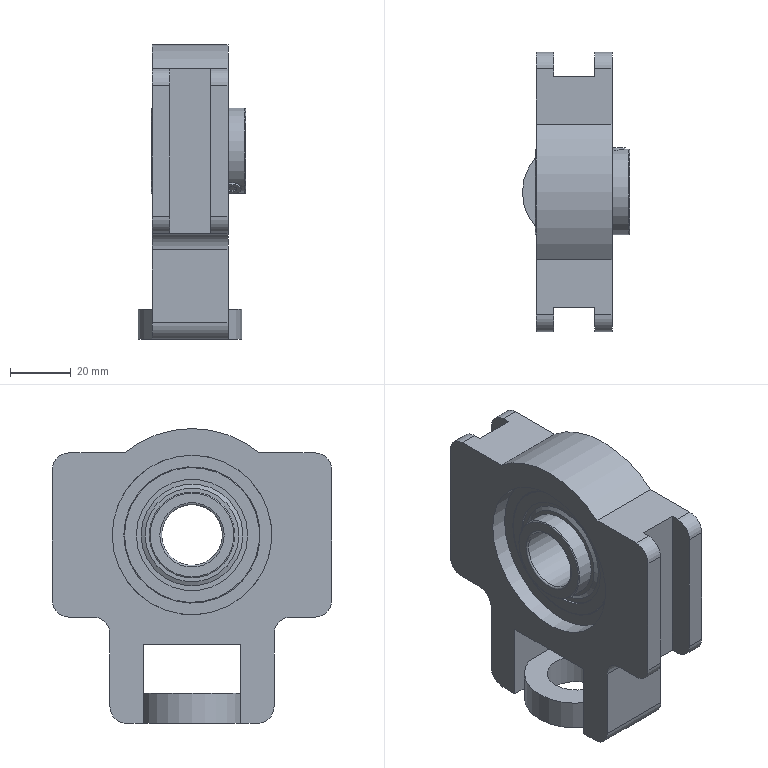Part | STEP file | TU_20_TF_2_14a | 10 solids | 221 faces | box 35.3 x 92 x 97 mm | volume 122603 mm3 | plane 114 | cylinder 87 | sphere 10 | torus 8 | cone 2 | commonest cylinder face diameters 0.275 x54 11 x12 28.2 x6 36.675 x4 6 x2 34 x2